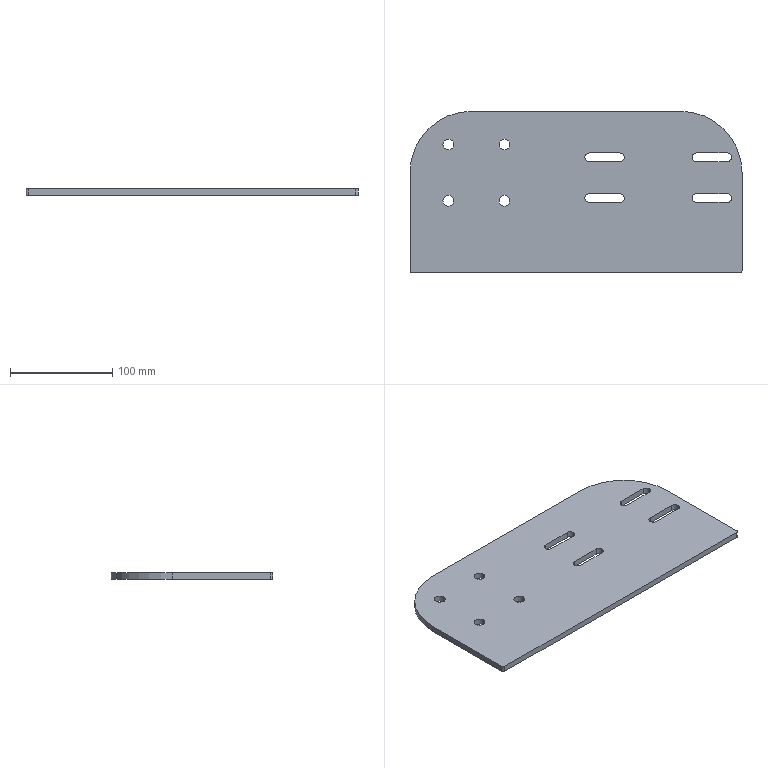Part | 1 solid | 38 faces | box 325 x 158 x 6 mm | volume 289259 mm3 | cylinder 24 | plane 14 | commonest cylinder face diameters 8.5 x12 10.5 x8 4 x2 120 x2
STEP:
#1=CARTESIAN_POINT('',(152.25,-25.,-3.));
#2=VERTEX_POINT('',#1);
#3=CARTESIAN_POINT('',(148.,-20.75,-3.));
#4=VERTEX_POINT('',#3);
#5=CARTESIAN_POINT('',(148.,-25.,-3.));
#6=DIRECTION('',(0.,0.,1.));
#7=DIRECTION('',(1.,0.,0.));
#8=AXIS2_PLACEMENT_3D('',#5,#6,#7);
#9=CIRCLE('',#8,4.25);
#10=EDGE_CURVE('',#2,#4,#9,.T.);
#11=ORIENTED_EDGE('',*,*,#10,.F.);
#12=CARTESIAN_POINT('',(152.25,-25.,3.));
#13=VERTEX_POINT('',#12);
#14=CARTESIAN_POINT('',(152.25,-25.,-3.));
#15=DIRECTION('',(0.,0.,1.));
#16=VECTOR('',#15,1000.);
#17=LINE('',#14,#16);
#18=EDGE_CURVE('',#2,#13,#17,.T.);
#19=ORIENTED_EDGE('',*,*,#18,.T.);
#20=CARTESIAN_POINT('',(148.,-20.75,3.));
#21=VERTEX_POINT('',#20);
#22=CARTESIAN_POINT('',(148.,-25.,3.));
#23=DIRECTION('',(0.,0.,1.));
#24=DIRECTION('',(1.,0.,0.));
#25=AXIS2_PLACEMENT_3D('',#22,#23,#24);
#26=CIRCLE('',#25,4.25);
#27=EDGE_CURVE('',#13,#21,#26,.T.);
#28=ORIENTED_EDGE('',*,*,#27,.T.);
#29=CARTESIAN_POINT('',(148.,-20.75,-3.));
#30=DIRECTION('',(0.,0.,1.));
#31=VECTOR('',#30,1000.);
#32=LINE('',#29,#31);
#33=EDGE_CURVE('',#4,#21,#32,.T.);
#34=ORIENTED_EDGE('',*,*,#33,.F.);
#35=EDGE_LOOP('',(#11,#19,#28,#34));
#36=FACE_OUTER_BOUND('',#35,.T.);
#37=CARTESIAN_POINT('',(148.,-25.,-3.));
#38=DIRECTION('',(0.,0.,1.));
#39=DIRECTION('',(1.,0.,0.));
#40=AXIS2_PLACEMENT_3D('',#37,#38,#39);
#41=CYLINDRICAL_SURFACE('',#40,4.25);
#42=ADVANCED_FACE('',(#36),#41,.F.);
#43=CARTESIAN_POINT('',(47.25,-25.,-3.));
#44=VERTEX_POINT('',#43);
#45=CARTESIAN_POINT('',(43.,-20.75,-3.));
#46=VERTEX_POINT('',#45);
#47=CARTESIAN_POINT('',(43.,-25.,-3.));
#48=DIRECTION('',(0.,0.,1.));
#49=DIRECTION('',(1.,0.,0.));
#50=AXIS2_PLACEMENT_3D('',#47,#48,#49);
#51=CIRCLE('',#50,4.25);
#52=EDGE_CURVE('',#44,#46,#51,.T.);
#53=ORIENTED_EDGE('',*,*,#52,.F.);
#54=CARTESIAN_POINT('',(47.25,-25.,3.));
#55=VERTEX_POINT('',#54);
#56=CARTESIAN_POINT('',(47.25,-25.,-3.));
#57=DIRECTION('',(0.,0.,1.));
#58=VECTOR('',#57,1000.);
#59=LINE('',#56,#58);
#60=EDGE_CURVE('',#44,#55,#59,.T.);
#61=ORIENTED_EDGE('',*,*,#60,.T.);
#62=CARTESIAN_POINT('',(43.,-20.75,3.));
#63=VERTEX_POINT('',#62);
#64=CARTESIAN_POINT('',(43.,-25.,3.));
#65=DIRECTION('',(0.,0.,1.));
#66=DIRECTION('',(1.,0.,0.));
#67=AXIS2_PLACEMENT_3D('',#64,#65,#66);
#68=CIRCLE('',#67,4.25);
#69=EDGE_CURVE('',#55,#63,#68,.T.);
#70=ORIENTED_EDGE('',*,*,#69,.T.);
#71=CARTESIAN_POINT('',(43.,-20.75,-3.));
#72=DIRECTION('',(0.,0.,1.));
#73=VECTOR('',#72,1000.);
#74=LINE('',#71,#73);
#75=EDGE_CURVE('',#46,#63,#74,.T.);
#76=ORIENTED_EDGE('',*,*,#75,.F.);
#77=EDGE_LOOP('',(#53,#61,#70,#76));
#78=FACE_OUTER_BOUND('',#77,.T.);
#79=CARTESIAN_POINT('',(43.,-25.,-3.));
#80=DIRECTION('',(0.,0.,1.));
#81=DIRECTION('',(1.,0.,0.));
#82=AXIS2_PLACEMENT_3D('',#79,#80,#81);
#83=CYLINDRICAL_SURFACE('',#82,4.25);
#84=ADVANCED_FACE('',(#78),#83,.F.);
#85=CARTESIAN_POINT('',(152.25,15.,-3.));
#86=VERTEX_POINT('',#85);
#87=CARTESIAN_POINT('',(148.,19.25,-3.));
#88=VERTEX_POINT('',#87);
#89=CARTESIAN_POINT('',(148.,15.,-3.));
#90=DIRECTION('',(0.,0.,1.));
#91=DIRECTION('',(1.,0.,0.));
#92=AXIS2_PLACEMENT_3D('',#89,#90,#91);
#93=CIRCLE('',#92,4.25);
#94=EDGE_CURVE('',#86,#88,#93,.T.);
#95=ORIENTED_EDGE('',*,*,#94,.F.);
#96=CARTESIAN_POINT('',(152.25,15.,3.));
#97=VERTEX_POINT('',#96);
#98=CARTESIAN_POINT('',(152.25,15.,-3.));
#99=DIRECTION('',(0.,0.,1.));
#100=VECTOR('',#99,1000.);
#101=LINE('',#98,#100);
#102=EDGE_CURVE('',#86,#97,#101,.T.);
#103=ORIENTED_EDGE('',*,*,#102,.T.);
#104=CARTESIAN_POINT('',(148.,19.25,3.));
#105=VERTEX_POINT('',#104);
#106=CARTESIAN_POINT('',(148.,15.,3.));
#107=DIRECTION('',(0.,0.,1.));
#108=DIRECTION('',(1.,0.,0.));
#109=AXIS2_PLACEMENT_3D('',#106,#107,#108);
#110=CIRCLE('',#109,4.25);
#111=EDGE_CURVE('',#97,#105,#110,.T.);
#112=ORIENTED_EDGE('',*,*,#111,.T.);
#113=CARTESIAN_POINT('',(148.,19.25,-3.));
#114=DIRECTION('',(0.,0.,1.));
#115=VECTOR('',#114,1000.);
#116=LINE('',#113,#115);
#117=EDGE_CURVE('',#88,#105,#116,.T.);
#118=ORIENTED_EDGE('',*,*,#117,.F.);
#119=EDGE_LOOP('',(#95,#103,#112,#118));
#120=FACE_OUTER_BOUND('',#119,.T.);
#121=CARTESIAN_POINT('',(148.,15.,-3.));
#122=DIRECTION('',(0.,0.,1.));
#123=DIRECTION('',(1.,0.,0.));
#124=AXIS2_PLACEMENT_3D('',#121,#122,#123);
#125=CYLINDRICAL_SURFACE('',#124,4.25);
#126=ADVANCED_FACE('',(#120),#125,.F.);
#127=CARTESIAN_POINT('',(47.25,15.,-3.));
#128=VERTEX_POINT('',#127);
#129=CARTESIAN_POINT('',(43.,19.25,-3.));
#130=VERTEX_POINT('',#129);
#131=CARTESIAN_POINT('',(43.,15.,-3.));
#132=DIRECTION('',(0.,0.,1.));
#133=DIRECTION('',(1.,0.,0.));
#134=AXIS2_PLACEMENT_3D('',#131,#132,#133);
#135=CIRCLE('',#134,4.25);
#136=EDGE_CURVE('',#128,#130,#135,.T.);
#137=ORIENTED_EDGE('',*,*,#136,.F.);
#138=CARTESIAN_POINT('',(47.25,15.,3.));
#139=VERTEX_POINT('',#138);
#140=CARTESIAN_POINT('',(47.25,15.,-3.));
#141=DIRECTION('',(0.,0.,1.));
#142=VECTOR('',#141,1000.);
#143=LINE('',#140,#142);
#144=EDGE_CURVE('',#128,#139,#143,.T.);
#145=ORIENTED_EDGE('',*,*,#144,.T.);
#146=CARTESIAN_POINT('',(43.,19.25,3.));
#147=VERTEX_POINT('',#146);
#148=CARTESIAN_POINT('',(43.,15.,3.));
#149=DIRECTION('',(0.,0.,1.));
#150=DIRECTION('',(1.,0.,0.));
#151=AXIS2_PLACEMENT_3D('',#148,#149,#150);
#152=CIRCLE('',#151,4.25);
#153=EDGE_CURVE('',#139,#147,#152,.T.);
#154=ORIENTED_EDGE('',*,*,#153,.T.);
#155=CARTESIAN_POINT('',(43.,19.25,-3.));
#156=DIRECTION('',(0.,0.,1.));
#157=VECTOR('',#156,1000.);
#158=LINE('',#155,#157);
#159=EDGE_CURVE('',#130,#147,#158,.T.);
#160=ORIENTED_EDGE('',*,*,#159,.F.);
#161=EDGE_LOOP('',(#137,#145,#154,#160));
#162=FACE_OUTER_BOUND('',#161,.T.);
#163=CARTESIAN_POINT('',(43.,15.,-3.));
#164=DIRECTION('',(0.,0.,1.));
#165=DIRECTION('',(1.,0.,0.));
#166=AXIS2_PLACEMENT_3D('',#163,#164,#165);
#167=CYLINDRICAL_SURFACE('',#166,4.25);
#168=ADVANCED_FACE('',(#162),#167,.F.);
#169=CARTESIAN_POINT('',(-75.25,-27.5,-3.));
#170=VERTEX_POINT('',#169);
#171=CARTESIAN_POINT('',(-64.75,-27.5,-3.));
#172=VERTEX_POINT('',#171);
#173=CARTESIAN_POINT('',(-70.,-27.5,-3.));
#174=DIRECTION('',(0.,0.,1.));
#175=DIRECTION('',(1.,0.,0.));
#176=AXIS2_PLACEMENT_3D('',#173,#174,#175);
#177=CIRCLE('',#176,5.25);
#178=EDGE_CURVE('',#170,#172,#177,.T.);
#179=ORIENTED_EDGE('',*,*,#178,.F.);
#180=CARTESIAN_POINT('',(-75.25,-27.5,3.));
#181=VERTEX_POINT('',#180);
#182=CARTESIAN_POINT('',(-75.25,-27.5,-3.));
#183=DIRECTION('',(0.,0.,1.));
#184=VECTOR('',#183,1000.);
#185=LINE('',#182,#184);
#186=EDGE_CURVE('',#170,#181,#185,.T.);
#187=ORIENTED_EDGE('',*,*,#186,.T.);
#188=CARTESIAN_POINT('',(-64.75,-27.5,3.));
#189=VERTEX_POINT('',#188);
#190=CARTESIAN_POINT('',(-70.,-27.5,3.));
#191=DIRECTION('',(0.,0.,1.));
#192=DIRECTION('',(1.,0.,0.));
#193=AXIS2_PLACEMENT_3D('',#190,#191,#192);
#194=CIRCLE('',#193,5.25);
#195=EDGE_CURVE('',#181,#189,#194,.T.);
#196=ORIENTED_EDGE('',*,*,#195,.T.);
#197=CARTESIAN_POINT('',(-64.75,-27.5,-3.));
#198=DIRECTION('',(0.,0.,1.));
#199=VECTOR('',#198,1000.);
#200=LINE('',#197,#199);
#201=EDGE_CURVE('',#172,#189,#200,.T.);
#202=ORIENTED_EDGE('',*,*,#201,.F.);
#203=EDGE_LOOP('',(#179,#187,#196,#202));
#204=FACE_OUTER_BOUND('',#203,.T.);
#205=CARTESIAN_POINT('',(-70.,-27.5,-3.));
#206=DIRECTION('',(0.,0.,1.));
#207=DIRECTION('',(1.,0.,0.));
#208=AXIS2_PLACEMENT_3D('',#205,#206,#207);
#209=CYLINDRICAL_SURFACE('',#208,5.25);
#210=ADVANCED_FACE('',(#204),#209,.F.);
#211=CARTESIAN_POINT('',(-130.25,-27.5,-3.));
#212=VERTEX_POINT('',#211);
#213=CARTESIAN_POINT('',(-119.75,-27.5,-3.));
#214=VERTEX_POINT('',#213);
#215=CARTESIAN_POINT('',(-125.,-27.5,-3.));
#216=DIRECTION('',(0.,0.,1.));
#217=DIRECTION('',(1.,0.,0.));
#218=AXIS2_PLACEMENT_3D('',#215,#216,#217);
#219=CIRCLE('',#218,5.25);
#220=EDGE_CURVE('',#212,#214,#219,.T.);
#221=ORIENTED_EDGE('',*,*,#220,.F.);
#222=CARTESIAN_POINT('',(-130.25,-27.5,3.));
#223=VERTEX_POINT('',#222);
#224=CARTESIAN_POINT('',(-130.25,-27.5,-3.));
#225=DIRECTION('',(0.,0.,1.));
#226=VECTOR('',#225,1000.);
#227=LINE('',#224,#226);
#228=EDGE_CURVE('',#212,#223,#227,.T.);
#229=ORIENTED_EDGE('',*,*,#228,.T.);
#230=CARTESIAN_POINT('',(-119.75,-27.5,3.));
#231=VERTEX_POINT('',#230);
#232=CARTESIAN_POINT('',(-125.,-27.5,3.));
#233=DIRECTION('',(0.,0.,1.));
#234=DIRECTION('',(1.,0.,0.));
#235=AXIS2_PLACEMENT_3D('',#232,#233,#234);
#236=CIRCLE('',#235,5.25);
#237=EDGE_CURVE('',#223,#231,#236,.T.);
#238=ORIENTED_EDGE('',*,*,#237,.T.);
#239=CARTESIAN_POINT('',(-119.75,-27.5,-3.));
#240=DIRECTION('',(0.,0.,1.));
#241=VECTOR('',#240,1000.);
#242=LINE('',#239,#241);
#243=EDGE_CURVE('',#214,#231,#242,.T.);
#244=ORIENTED_EDGE('',*,*,#243,.F.);
#245=EDGE_LOOP('',(#221,#229,#238,#244));
#246=FACE_OUTER_BOUND('',#245,.T.);
#247=CARTESIAN_POINT('',(-125.,-27.5,-3.));
#248=DIRECTION('',(0.,0.,1.));
#249=DIRECTION('',(1.,0.,0.));
#250=AXIS2_PLACEMENT_3D('',#247,#248,#249);
#251=CYLINDRICAL_SURFACE('',#250,5.25);
#252=ADVANCED_FACE('',(#246),#251,.F.);
#253=CARTESIAN_POINT('',(-75.25,27.5,-3.));
#254=VERTEX_POINT('',#253);
#255=CARTESIAN_POINT('',(-64.75,27.5,-3.));
#256=VERTEX_POINT('',#255);
#257=CARTESIAN_POINT('',(-70.,27.5,-3.));
#258=DIRECTION('',(0.,0.,1.));
#259=DIRECTION('',(1.,0.,0.));
#260=AXIS2_PLACEMENT_3D('',#257,#258,#259);
#261=CIRCLE('',#260,5.25);
#262=EDGE_CURVE('',#254,#256,#261,.T.);
#263=ORIENTED_EDGE('',*,*,#262,.F.);
#264=CARTESIAN_POINT('',(-75.25,27.5,3.));
#265=VERTEX_POINT('',#264);
#266=CARTESIAN_POINT('',(-75.25,27.5,-3.));
#267=DIRECTION('',(0.,0.,1.));
#268=VECTOR('',#267,1000.);
#269=LINE('',#266,#268);
#270=EDGE_CURVE('',#254,#265,#269,.T.);
#271=ORIENTED_EDGE('',*,*,#270,.T.);
#272=CARTESIAN_POINT('',(-64.75,27.5,3.));
#273=VERTEX_POINT('',#272);
#274=CARTESIAN_POINT('',(-70.,27.5,3.));
#275=DIRECTION('',(0.,0.,1.));
#276=DIRECTION('',(1.,0.,0.));
#277=AXIS2_PLACEMENT_3D('',#274,#275,#276);
#278=CIRCLE('',#277,5.25);
#279=EDGE_CURVE('',#265,#273,#278,.T.);
#280=ORIENTED_EDGE('',*,*,#279,.T.);
#281=CARTESIAN_POINT('',(-64.75,27.5,-3.));
#282=DIRECTION('',(0.,0.,1.));
#283=VECTOR('',#282,1000.);
#284=LINE('',#281,#283);
#285=EDGE_CURVE('',#256,#273,#284,.T.);
#286=ORIENTED_EDGE('',*,*,#285,.F.);
#287=EDGE_LOOP('',(#263,#271,#280,#286));
#288=FACE_OUTER_BOUND('',#287,.T.);
#289=CARTESIAN_POINT('',(-70.,27.5,-3.));
#290=DIRECTION('',(0.,0.,1.));
#291=DIRECTION('',(1.,0.,0.));
#292=AXIS2_PLACEMENT_3D('',#289,#290,#291);
#293=CYLINDRICAL_SURFACE('',#292,5.25);
#294=ADVANCED_FACE('',(#288),#293,.F.);
#295=CARTESIAN_POINT('',(-130.25,27.5,-3.));
#296=VERTEX_POINT('',#295);
#297=CARTESIAN_POINT('',(-119.75,27.5,-3.));
#298=VERTEX_POINT('',#297);
#299=CARTESIAN_POINT('',(-125.,27.5,-3.));
#300=DIRECTION('',(0.,0.,1.));
#301=DIRECTION('',(1.,0.,0.));
#302=AXIS2_PLACEMENT_3D('',#299,#300,#301);
#303=CIRCLE('',#302,5.25);
#304=EDGE_CURVE('',#296,#298,#303,.T.);
#305=ORIENTED_EDGE('',*,*,#304,.F.);
#306=CARTESIAN_POINT('',(-130.25,27.5,3.));
#307=VERTEX_POINT('',#306);
#308=CARTESIAN_POINT('',(-130.25,27.5,-3.));
#309=DIRECTION('',(0.,0.,1.));
#310=VECTOR('',#309,1000.);
#311=LINE('',#308,#310);
#312=EDGE_CURVE('',#296,#307,#311,.T.);
#313=ORIENTED_EDGE('',*,*,#312,.T.);
#314=CARTESIAN_POINT('',(-119.75,27.5,3.));
#315=VERTEX_POINT('',#314);
#316=CARTESIAN_POINT('',(-125.,27.5,3.));
#317=DIRECTION('',(0.,0.,1.));
#318=DIRECTION('',(1.,0.,0.));
#319=AXIS2_PLACEMENT_3D('',#316,#317,#318);
#320=CIRCLE('',#319,5.25);
#321=EDGE_CURVE('',#307,#315,#320,.T.);
#322=ORIENTED_EDGE('',*,*,#321,.T.);
#323=CARTESIAN_POINT('',(-119.75,27.5,-3.));
#324=DIRECTION('',(0.,0.,1.));
#325=VECTOR('',#324,1000.);
#326=LINE('',#323,#325);
#327=EDGE_CURVE('',#298,#315,#326,.T.);
#328=ORIENTED_EDGE('',*,*,#327,.F.);
#329=EDGE_LOOP('',(#305,#313,#322,#328));
#330=FACE_OUTER_BOUND('',#329,.T.);
#331=CARTESIAN_POINT('',(-125.,27.5,-3.));
#332=DIRECTION('',(0.,0.,1.));
#333=DIRECTION('',(1.,0.,0.));
#334=AXIS2_PLACEMENT_3D('',#331,#332,#333);
#335=CYLINDRICAL_SURFACE('',#334,5.25);
#336=ADVANCED_FACE('',(#330),#335,.F.);
#337=CARTESIAN_POINT('',(-162.5,0.,-3.));
#338=VERTEX_POINT('',#337);
#339=CARTESIAN_POINT('',(-162.5,0.,3.));
#340=VERTEX_POINT('',#339);
#341=CARTESIAN_POINT('',(-162.5,0.,-3.));
#342=DIRECTION('',(0.,0.,1.));
#343=VECTOR('',#342,1000.);
#344=LINE('',#341,#343);
#345=EDGE_CURVE('',#338,#340,#344,.T.);
#346=ORIENTED_EDGE('',*,*,#345,.T.);
#347=CARTESIAN_POINT('',(-102.5,60.,3.));
#348=VERTEX_POINT('',#347);
#349=CARTESIAN_POINT('',(-102.5,0.,3.));
#350=DIRECTION('',(0.,0.,1.));
#351=DIRECTION('',(1.,0.,0.));
#352=AXIS2_PLACEMENT_3D('',#349,#350,#351);
#353=CIRCLE('',#352,60.);
#354=EDGE_CURVE('',#348,#340,#353,.T.);
#355=ORIENTED_EDGE('',*,*,#354,.F.);
#356=CARTESIAN_POINT('',(-102.5,60.,-3.));
#357=VERTEX_POINT('',#356);
#358=CARTESIAN_POINT('',(-102.5,60.,3.));
#359=DIRECTION('',(0.,0.,-1.));
#360=VECTOR('',#359,1000.);
#361=LINE('',#358,#360);
#362=EDGE_CURVE('',#348,#357,#361,.T.);
#363=ORIENTED_EDGE('',*,*,#362,.T.);
#364=CARTESIAN_POINT('',(-102.5,0.,-3.));
#365=DIRECTION('',(0.,0.,1.));
#366=DIRECTION('',(1.,0.,0.));
#367=AXIS2_PLACEMENT_3D('',#364,#365,#366);
#368=CIRCLE('',#367,60.);
#369=EDGE_CURVE('',#357,#338,#368,.T.);
#370=ORIENTED_EDGE('',*,*,#369,.T.);
#371=EDGE_LOOP('',(#346,#355,#363,#370));
#372=FACE_OUTER_BOUND('',#371,.T.);
#373=CARTESIAN_POINT('',(-102.5,0.,3.));
#374=DIRECTION('',(0.,0.,-1.));
#375=DIRECTION('',(-1.,0.,0.));
#376=AXIS2_PLACEMENT_3D('',#373,#374,#375);
#377=CYLINDRICAL_SURFACE('',#376,60.);
#378=ADVANCED_FACE('',(#372),#377,.T.);
#379=CARTESIAN_POINT('',(162.5,0.,3.));
#380=VERTEX_POINT('',#379);
#381=CARTESIAN_POINT('',(102.5,60.,3.));
#382=VERTEX_POINT('',#381);
#383=CARTESIAN_POINT('',(102.5,0.,3.));
#384=DIRECTION('',(0.,0.,1.));
#385=DIRECTION('',(1.,0.,0.));
#386=AXIS2_PLACEMENT_3D('',#383,#384,#385);
#387=CIRCLE('',#386,60.);
#388=EDGE_CURVE('',#380,#382,#387,.T.);
#389=ORIENTED_EDGE('',*,*,#388,.F.);
#390=CARTESIAN_POINT('',(162.5,0.,-3.));
#391=VERTEX_POINT('',#390);
#392=CARTESIAN_POINT('',(162.5,0.,-3.));
#393=DIRECTION('',(0.,0.,1.));
#394=VECTOR('',#393,1000.);
#395=LINE('',#392,#394);
#396=EDGE_CURVE('',#391,#380,#395,.T.);
#397=ORIENTED_EDGE('',*,*,#396,.F.);
#398=CARTESIAN_POINT('',(102.5,60.,-3.));
#399=VERTEX_POINT('',#398);
#400=CARTESIAN_POINT('',(102.5,0.,-3.));
#401=DIRECTION('',(0.,0.,1.));
#402=DIRECTION('',(1.,0.,0.));
#403=AXIS2_PLACEMENT_3D('',#400,#401,#402);
#404=CIRCLE('',#403,60.);
#405=EDGE_CURVE('',#391,#399,#404,.T.);
#406=ORIENTED_EDGE('',*,*,#405,.T.);
#407=CARTESIAN_POINT('',(102.5,60.,3.));
#408=DIRECTION('',(0.,0.,-1.));
#409=VECTOR('',#408,1000.);
#410=LINE('',#407,#409);
#411=EDGE_CURVE('',#382,#399,#410,.T.);
#412=ORIENTED_EDGE('',*,*,#411,.F.);
#413=EDGE_LOOP('',(#389,#397,#406,#412));
#414=FACE_OUTER_BOUND('',#413,.T.);
#415=CARTESIAN_POINT('',(102.5,0.,3.));
#416=DIRECTION('',(0.,0.,-1.));
#417=DIRECTION('',(-1.,0.,0.));
#418=AXIS2_PLACEMENT_3D('',#415,#416,#417);
#419=CYLINDRICAL_SURFACE('',#418,60.);
#420=ADVANCED_FACE('',(#414),#419,.T.);
#421=CARTESIAN_POINT('',(-102.5,60.,-3.));
#422=DIRECTION('',(-1.,0.,0.));
#423=VECTOR('',#422,1000.);
#424=LINE('',#421,#423);
#425=EDGE_CURVE('',#399,#357,#424,.T.);
#426=ORIENTED_EDGE('',*,*,#425,.T.);
#427=ORIENTED_EDGE('',*,*,#362,.F.);
#428=CARTESIAN_POINT('',(-102.5,60.,3.));
#429=DIRECTION('',(-1.,0.,0.));
#430=VECTOR('',#429,1000.);
#431=LINE('',#428,#430);
#432=EDGE_CURVE('',#382,#348,#431,.T.);
#433=ORIENTED_EDGE('',*,*,#432,.F.);
#434=ORIENTED_EDGE('',*,*,#411,.T.);
#435=EDGE_LOOP('',(#426,#427,#433,#434));
#436=FACE_OUTER_BOUND('',#435,.T.);
#437=CARTESIAN_POINT('',(-102.5,60.,3.));
#438=DIRECTION('',(0.,-1.,0.));
#439=DIRECTION('',(1.,0.,0.));
#440=AXIS2_PLACEMENT_3D('',#437,#438,#439);
#441=PLANE('',#440);
#442=ADVANCED_FACE('',(#436),#441,.F.);
#443=CARTESIAN_POINT('',(118.,-20.75,3.));
#444=VERTEX_POINT('',#443);
#445=CARTESIAN_POINT('',(118.,-29.25,3.));
#446=VERTEX_POINT('',#445);
#447=CARTESIAN_POINT('',(118.,-25.,3.));
#448=DIRECTION('',(0.,0.,1.));
#449=DIRECTION('',(1.,0.,0.));
#450=AXIS2_PLACEMENT_3D('',#447,#448,#449);
#451=CIRCLE('',#450,4.25);
#452=EDGE_CURVE('',#444,#446,#451,.T.);
#453=ORIENTED_EDGE('',*,*,#452,.F.);
#454=CARTESIAN_POINT('',(118.,-20.75,3.));
#455=DIRECTION('',(-1.,0.,0.));
#456=VECTOR('',#455,1000.);
#457=LINE('',#454,#456);
#458=EDGE_CURVE('',#21,#444,#457,.T.);
#459=ORIENTED_EDGE('',*,*,#458,.F.);
#460=ORIENTED_EDGE('',*,*,#27,.F.);
#461=CARTESIAN_POINT('',(148.,-29.25,3.));
#462=VERTEX_POINT('',#461);
#463=CARTESIAN_POINT('',(148.,-25.,3.));
#464=DIRECTION('',(0.,0.,1.));
#465=DIRECTION('',(1.,0.,0.));
#466=AXIS2_PLACEMENT_3D('',#463,#464,#465);
#467=CIRCLE('',#466,4.25);
#468=EDGE_CURVE('',#462,#13,#467,.T.);
#469=ORIENTED_EDGE('',*,*,#468,.F.);
#470=CARTESIAN_POINT('',(118.,-29.25,3.));
#471=DIRECTION('',(1.,0.,0.));
#472=VECTOR('',#471,1000.);
#473=LINE('',#470,#472);
#474=EDGE_CURVE('',#446,#462,#473,.T.);
#475=ORIENTED_EDGE('',*,*,#474,.F.);
#476=EDGE_LOOP('',(#453,#459,#460,#469,#475));
#477=FACE_BOUND('',#476,.T.);
#478=CARTESIAN_POINT('',(13.,-20.75,3.));
#479=VERTEX_POINT('',#478);
#480=CARTESIAN_POINT('',(13.,-29.25,3.));
#481=VERTEX_POINT('',#480);
#482=CARTESIAN_POINT('',(13.,-25.,3.));
#483=DIRECTION('',(0.,0.,1.));
#484=DIRECTION('',(1.,0.,0.));
#485=AXIS2_PLACEMENT_3D('',#482,#483,#484);
#486=CIRCLE('',#485,4.25);
#487=EDGE_CURVE('',#479,#481,#486,.T.);
#488=ORIENTED_EDGE('',*,*,#487,.F.);
#489=CARTESIAN_POINT('',(13.,-20.75,3.));
#490=DIRECTION('',(-1.,0.,0.));
#491=VECTOR('',#490,1000.);
#492=LINE('',#489,#491);
#493=EDGE_CURVE('',#63,#479,#492,.T.);
#494=ORIENTED_EDGE('',*,*,#493,.F.);
#495=ORIENTED_EDGE('',*,*,#69,.F.);
#496=CARTESIAN_POINT('',(43.,-29.25,3.));
#497=VERTEX_POINT('',#496);
#498=CARTESIAN_POINT('',(43.,-25.,3.));
#499=DIRECTION('',(0.,0.,1.));
#500=DIRECTION('',(1.,0.,0.));
#501=AXIS2_PLACEMENT_3D('',#498,#499,#500);
#502=CIRCLE('',#501,4.25);
#503=EDGE_CURVE('',#497,#55,#502,.T.);
#504=ORIENTED_EDGE('',*,*,#503,.F.);
#505=CARTESIAN_POINT('',(13.,-29.25,3.));
#506=DIRECTION('',(1.,0.,0.));
#507=VECTOR('',#506,1000.);
#508=LINE('',#505,#507);
#509=EDGE_CURVE('',#481,#497,#508,.T.);
#510=ORIENTED_EDGE('',*,*,#509,.F.);
#511=EDGE_LOOP('',(#488,#494,#495,#504,#510));
#512=FACE_BOUND('',#511,.T.);
#513=CARTESIAN_POINT('',(118.,19.25,3.));
#514=VERTEX_POINT('',#513);
#515=CARTESIAN_POINT('',(118.,10.75,3.));
#516=VERTEX_POINT('',#515);
#517=CARTESIAN_POINT('',(118.,15.,3.));
#518=DIRECTION('',(0.,0.,1.));
#519=DIRECTION('',(1.,0.,0.));
#520=AXIS2_PLACEMENT_3D('',#517,#518,#519);
#521=CIRCLE('',#520,4.25);
#522=EDGE_CURVE('',#514,#516,#521,.T.);
#523=ORIENTED_EDGE('',*,*,#522,.F.);
#524=CARTESIAN_POINT('',(118.,19.25,3.));
#525=DIRECTION('',(-1.,0.,0.));
#526=VECTOR('',#525,1000.);
#527=LINE('',#524,#526);
#528=EDGE_CURVE('',#105,#514,#527,.T.);
#529=ORIENTED_EDGE('',*,*,#528,.F.);
#530=ORIENTED_EDGE('',*,*,#111,.F.);
#531=CARTESIAN_POINT('',(148.,10.75,3.));
#532=VERTEX_POINT('',#531);
#533=CARTESIAN_POINT('',(148.,15.,3.));
#534=DIRECTION('',(0.,0.,1.));
#535=DIRECTION('',(1.,0.,0.));
#536=AXIS2_PLACEMENT_3D('',#533,#534,#535);
#537=CIRCLE('',#536,4.25);
#538=EDGE_CURVE('',#532,#97,#537,.T.);
#539=ORIENTED_EDGE('',*,*,#538,.F.);
#540=CARTESIAN_POINT('',(118.,10.75,3.));
#541=DIRECTION('',(1.,0.,0.));
#542=VECTOR('',#541,1000.);
#543=LINE('',#540,#542);
#544=EDGE_CURVE('',#516,#532,#543,.T.);
#545=ORIENTED_EDGE('',*,*,#544,.F.);
#546=EDGE_LOOP('',(#523,#529,#530,#539,#545));
#547=FACE_BOUND('',#546,.T.);
#548=CARTESIAN_POINT('',(13.,19.25,3.));
#549=VERTEX_POINT('',#548);
#550=CARTESIAN_POINT('',(13.,10.75,3.));
#551=VERTEX_POINT('',#550);
#552=CARTESIAN_POINT('',(13.,15.,3.));
#553=DIRECTION('',(0.,0.,1.));
#554=DIRECTION('',(1.,0.,0.));
#555=AXIS2_PLACEMENT_3D('',#552,#553,#554);
#556=CIRCLE('',#555,4.25);
#557=EDGE_CURVE('',#549,#551,#556,.T.);
#558=ORIENTED_EDGE('',*,*,#557,.F.);
#559=CARTESIAN_POINT('',(13.,19.25,3.));
#560=DIRECTION('',(-1.,0.,0.));
#561=VECTOR('',#560,1000.);
#562=LINE('',#559,#561);
#563=EDGE_CURVE('',#147,#549,#562,.T.);
#564=ORIENTED_EDGE('',*,*,#563,.F.);
#565=ORIENTED_EDGE('',*,*,#153,.F.);
#566=CARTESIAN_POINT('',(43.,10.75,3.));
#567=VERTEX_POINT('',#566);
#568=CARTESIAN_POINT('',(43.,15.,3.));
#569=DIRECTION('',(0.,0.,1.));
#570=DIRECTION('',(1.,0.,0.));
#571=AXIS2_PLACEMENT_3D('',#568,#569,#570);
#572=CIRCLE('',#571,4.25);
#573=EDGE_CURVE('',#567,#139,#572,.T.);
#574=ORIENTED_EDGE('',*,*,#573,.F.);
#575=CARTESIAN_POINT('',(13.,10.75,3.));
#576=DIRECTION('',(1.,0.,0.));
#577=VECTOR('',#576,1000.);
#578=LINE('',#575,#577);
#579=EDGE_CURVE('',#551,#567,#578,.T.);
#580=ORIENTED_EDGE('',*,*,#579,.F.);
#581=EDGE_LOOP('',(#558,#564,#565,#574,#580));
#582=FACE_BOUND('',#581,.T.);
#583=CARTESIAN_POINT('',(-70.,-27.5,3.));
#584=DIRECTION('',(0.,0.,1.));
#585=DIRECTION('',(1.,0.,0.));
#586=AXIS2_PLACEMENT_3D('',#583,#584,#585);
#587=CIRCLE('',#586,5.25);
#588=EDGE_CURVE('',#189,#181,#587,.T.);
#589=ORIENTED_EDGE('',*,*,#588,.F.);
#590=ORIENTED_EDGE('',*,*,#195,.F.);
#591=EDGE_LOOP('',(#589,#590));
#592=FACE_BOUND('',#591,.T.);
#593=CARTESIAN_POINT('',(-125.,-27.5,3.));
#594=DIRECTION('',(0.,0.,1.));
#595=DIRECTION('',(1.,0.,0.));
#596=AXIS2_PLACEMENT_3D('',#593,#594,#595);
#597=CIRCLE('',#596,5.25);
#598=EDGE_CURVE('',#231,#223,#597,.T.);
#599=ORIENTED_EDGE('',*,*,#598,.F.);
#600=ORIENTED_EDGE('',*,*,#237,.F.);
#601=EDGE_LOOP('',(#599,#600));
#602=FACE_BOUND('',#601,.T.);
#603=CARTESIAN_POINT('',(-70.,27.5,3.));
#604=DIRECTION('',(0.,0.,1.));
#605=DIRECTION('',(1.,0.,0.));
#606=AXIS2_PLACEMENT_3D('',#603,#604,#605);
#607=CIRCLE('',#606,5.25);
#608=EDGE_CURVE('',#273,#265,#607,.T.);
#609=ORIENTED_EDGE('',*,*,#608,.F.);
#610=ORIENTED_EDGE('',*,*,#279,.F.);
#611=EDGE_LOOP('',(#609,#610));
#612=FACE_BOUND('',#611,.T.);
#613=CARTESIAN_POINT('',(-125.,27.5,3.));
#614=DIRECTION('',(0.,0.,1.));
#615=DIRECTION('',(1.,0.,0.));
#616=AXIS2_PLACEMENT_3D('',#613,#614,#615);
#617=CIRCLE('',#616,5.25);
#618=EDGE_CURVE('',#315,#307,#617,.T.);
#619=ORIENTED_EDGE('',*,*,#618,.F.);
#620=ORIENTED_EDGE('',*,*,#321,.F.);
#621=EDGE_LOOP('',(#619,#620));
#622=FACE_BOUND('',#621,.T.);
#623=CARTESIAN_POINT('',(160.5,-98.,3.));
#624=VERTEX_POINT('',#623);
#625=CARTESIAN_POINT('',(-160.5,-98.,3.));
#626=VERTEX_POINT('',#625);
#627=CARTESIAN_POINT('',(0.,-98.,3.));
#628=DIRECTION('',(-1.,0.,0.));
#629=VECTOR('',#628,1000.);
#630=LINE('',#627,#629);
#631=EDGE_CURVE('',#624,#626,#630,.T.);
#632=ORIENTED_EDGE('',*,*,#631,.F.);
#633=CARTESIAN_POINT('',(162.5,-96.,3.));
#634=VERTEX_POINT('',#633);
#635=CARTESIAN_POINT('',(160.5,-96.,3.));
#636=DIRECTION('',(0.,0.,1.));
#637=DIRECTION('',(1.,0.,0.));
#638=AXIS2_PLACEMENT_3D('',#635,#636,#637);
#639=CIRCLE('',#638,2.);
#640=EDGE_CURVE('',#624,#634,#639,.T.);
#641=ORIENTED_EDGE('',*,*,#640,.T.);
#642=CARTESIAN_POINT('',(162.5,0.,3.));
#643=DIRECTION('',(0.,-1.,0.));
#644=VECTOR('',#643,1000.);
#645=LINE('',#642,#644);
#646=EDGE_CURVE('',#380,#634,#645,.T.);
#647=ORIENTED_EDGE('',*,*,#646,.F.);
#648=ORIENTED_EDGE('',*,*,#388,.T.);
#649=ORIENTED_EDGE('',*,*,#432,.T.);
#650=ORIENTED_EDGE('',*,*,#354,.T.);
#651=CARTESIAN_POINT('',(-162.5,-96.,3.));
#652=VERTEX_POINT('',#651);
#653=CARTESIAN_POINT('',(-162.5,0.,3.));
#654=DIRECTION('',(0.,1.,0.));
#655=VECTOR('',#654,1000.);
#656=LINE('',#653,#655);
#657=EDGE_CURVE('',#652,#340,#656,.T.);
#658=ORIENTED_EDGE('',*,*,#657,.F.);
#659=CARTESIAN_POINT('',(-160.5,-96.,3.));
#660=DIRECTION('',(0.,0.,1.));
#661=DIRECTION('',(1.,0.,0.));
#662=AXIS2_PLACEMENT_3D('',#659,#660,#661);
#663=CIRCLE('',#662,2.);
#664=EDGE_CURVE('',#652,#626,#663,.T.);
#665=ORIENTED_EDGE('',*,*,#664,.T.);
#666=EDGE_LOOP('',(#632,#641,#647,#648,#649,#650,#658,#665));
#667=FACE_OUTER_BOUND('',#666,.T.);
#668=CARTESIAN_POINT('',(-102.5,0.,3.));
#669=DIRECTION('',(0.,0.,1.));
#670=DIRECTION('',(1.,0.,0.));
#671=AXIS2_PLACEMENT_3D('',#668,#669,#670);
#672=PLANE('',#671);
#673=ADVANCED_FACE('',(#477,#512,#547,#582,#592,#602,#612,#622,#667),#672,.T.);
#674=CARTESIAN_POINT('',(118.,-20.75,-3.));
#675=VERTEX_POINT('',#674);
#676=CARTESIAN_POINT('',(118.,-20.75,-3.));
#677=DIRECTION('',(-1.,0.,0.));
#678=VECTOR('',#677,1000.);
#679=LINE('',#676,#678);
#680=EDGE_CURVE('',#4,#675,#679,.T.);
#681=ORIENTED_EDGE('',*,*,#680,.T.);
#682=CARTESIAN_POINT('',(118.,-29.25,-3.));
#683=VERTEX_POINT('',#682);
#684=CARTESIAN_POINT('',(118.,-25.,-3.));
#685=DIRECTION('',(0.,0.,1.));
#686=DIRECTION('',(1.,0.,0.));
#687=AXIS2_PLACEMENT_3D('',#684,#685,#686);
#688=CIRCLE('',#687,4.25);
#689=EDGE_CURVE('',#675,#683,#688,.T.);
#690=ORIENTED_EDGE('',*,*,#689,.T.);
#691=CARTESIAN_POINT('',(148.,-29.25,-3.));
#692=VERTEX_POINT('',#691);
#693=CARTESIAN_POINT('',(118.,-29.25,-3.));
#694=DIRECTION('',(1.,0.,0.));
#695=VECTOR('',#694,1000.);
#696=LINE('',#693,#695);
#697=EDGE_CURVE('',#683,#692,#696,.T.);
#698=ORIENTED_EDGE('',*,*,#697,.T.);
#699=CARTESIAN_POINT('',(148.,-25.,-3.));
#700=DIRECTION('',(0.,0.,1.));
#701=DIRECTION('',(1.,0.,0.));
#702=AXIS2_PLACEMENT_3D('',#699,#700,#701);
#703=CIRCLE('',#702,4.25);
#704=EDGE_CURVE('',#692,#2,#703,.T.);
#705=ORIENTED_EDGE('',*,*,#704,.T.);
#706=ORIENTED_EDGE('',*,*,#10,.T.);
#707=EDGE_LOOP('',(#681,#690,#698,#705,#706));
#708=FACE_BOUND('',#707,.T.);
#709=CARTESIAN_POINT('',(13.,-20.75,-3.));
#710=VERTEX_POINT('',#709);
#711=CARTESIAN_POINT('',(13.,-20.75,-3.));
#712=DIRECTION('',(-1.,0.,0.));
#713=VECTOR('',#712,1000.);
#714=LINE('',#711,#713);
#715=EDGE_CURVE('',#46,#710,#714,.T.);
#716=ORIENTED_EDGE('',*,*,#715,.T.);
#717=CARTESIAN_POINT('',(13.,-29.25,-3.));
#718=VERTEX_POINT('',#717);
#719=CARTESIAN_POINT('',(13.,-25.,-3.));
#720=DIRECTION('',(0.,0.,1.));
#721=DIRECTION('',(1.,0.,0.));
#722=AXIS2_PLACEMENT_3D('',#719,#720,#721);
#723=CIRCLE('',#722,4.25);
#724=EDGE_CURVE('',#710,#718,#723,.T.);
#725=ORIENTED_EDGE('',*,*,#724,.T.);
#726=CARTESIAN_POINT('',(43.,-29.25,-3.));
#727=VERTEX_POINT('',#726);
#728=CARTESIAN_POINT('',(13.,-29.25,-3.));
#729=DIRECTION('',(1.,0.,0.));
#730=VECTOR('',#729,1000.);
#731=LINE('',#728,#730);
#732=EDGE_CURVE('',#718,#727,#731,.T.);
#733=ORIENTED_EDGE('',*,*,#732,.T.);
#734=CARTESIAN_POINT('',(43.,-25.,-3.));
#735=DIRECTION('',(0.,0.,1.));
#736=DIRECTION('',(1.,0.,0.));
#737=AXIS2_PLACEMENT_3D('',#734,#735,#736);
#738=CIRCLE('',#737,4.25);
#739=EDGE_CURVE('',#727,#44,#738,.T.);
#740=ORIENTED_EDGE('',*,*,#739,.T.);
#741=ORIENTED_EDGE('',*,*,#52,.T.);
#742=EDGE_LOOP('',(#716,#725,#733,#740,#741));
#743=FACE_BOUND('',#742,.T.);
#744=CARTESIAN_POINT('',(118.,19.25,-3.));
#745=VERTEX_POINT('',#744);
#746=CARTESIAN_POINT('',(118.,19.25,-3.));
#747=DIRECTION('',(-1.,0.,0.));
#748=VECTOR('',#747,1000.);
#749=LINE('',#746,#748);
#750=EDGE_CURVE('',#88,#745,#749,.T.);
#751=ORIENTED_EDGE('',*,*,#750,.T.);
#752=CARTESIAN_POINT('',(118.,10.75,-3.));
#753=VERTEX_POINT('',#752);
#754=CARTESIAN_POINT('',(118.,15.,-3.));
#755=DIRECTION('',(0.,0.,1.));
#756=DIRECTION('',(1.,0.,0.));
#757=AXIS2_PLACEMENT_3D('',#754,#755,#756);
#758=CIRCLE('',#757,4.25);
#759=EDGE_CURVE('',#745,#753,#758,.T.);
#760=ORIENTED_EDGE('',*,*,#759,.T.);
#761=CARTESIAN_POINT('',(148.,10.75,-3.));
#762=VERTEX_POINT('',#761);
#763=CARTESIAN_POINT('',(118.,10.75,-3.));
#764=DIRECTION('',(1.,0.,0.));
#765=VECTOR('',#764,1000.);
#766=LINE('',#763,#765);
#767=EDGE_CURVE('',#753,#762,#766,.T.);
#768=ORIENTED_EDGE('',*,*,#767,.T.);
#769=CARTESIAN_POINT('',(148.,15.,-3.));
#770=DIRECTION('',(0.,0.,1.));
#771=DIRECTION('',(1.,0.,0.));
#772=AXIS2_PLACEMENT_3D('',#769,#770,#771);
#773=CIRCLE('',#772,4.25);
#774=EDGE_CURVE('',#762,#86,#773,.T.);
#775=ORIENTED_EDGE('',*,*,#774,.T.);
#776=ORIENTED_EDGE('',*,*,#94,.T.);
#777=EDGE_LOOP('',(#751,#760,#768,#775,#776));
#778=FACE_BOUND('',#777,.T.);
#779=CARTESIAN_POINT('',(13.,19.25,-3.));
#780=VERTEX_POINT('',#779);
#781=CARTESIAN_POINT('',(13.,19.25,-3.));
#782=DIRECTION('',(-1.,0.,0.));
#783=VECTOR('',#782,1000.);
#784=LINE('',#781,#783);
#785=EDGE_CURVE('',#130,#780,#784,.T.);
#786=ORIENTED_EDGE('',*,*,#785,.T.);
#787=CARTESIAN_POINT('',(13.,10.75,-3.));
#788=VERTEX_POINT('',#787);
#789=CARTESIAN_POINT('',(13.,15.,-3.));
#790=DIRECTION('',(0.,0.,1.));
#791=DIRECTION('',(1.,0.,0.));
#792=AXIS2_PLACEMENT_3D('',#789,#790,#791);
#793=CIRCLE('',#792,4.25);
#794=EDGE_CURVE('',#780,#788,#793,.T.);
#795=ORIENTED_EDGE('',*,*,#794,.T.);
#796=CARTESIAN_POINT('',(43.,10.75,-3.));
#797=VERTEX_POINT('',#796);
#798=CARTESIAN_POINT('',(13.,10.75,-3.));
#799=DIRECTION('',(1.,0.,0.));
#800=VECTOR('',#799,1000.);
#801=LINE('',#798,#800);
#802=EDGE_CURVE('',#788,#797,#801,.T.);
#803=ORIENTED_EDGE('',*,*,#802,.T.);
#804=CARTESIAN_POINT('',(43.,15.,-3.));
#805=DIRECTION('',(0.,0.,1.));
#806=DIRECTION('',(1.,0.,0.));
#807=AXIS2_PLACEMENT_3D('',#804,#805,#806);
#808=CIRCLE('',#807,4.25);
#809=EDGE_CURVE('',#797,#128,#808,.T.);
#810=ORIENTED_EDGE('',*,*,#809,.T.);
#811=ORIENTED_EDGE('',*,*,#136,.T.);
#812=EDGE_LOOP('',(#786,#795,#803,#810,#811));
#813=FACE_BOUND('',#812,.T.);
#814=CARTESIAN_POINT('',(-70.,-27.5,-3.));
#815=DIRECTION('',(0.,0.,1.));
#816=DIRECTION('',(1.,0.,0.));
#817=AXIS2_PLACEMENT_3D('',#814,#815,#816);
#818=CIRCLE('',#817,5.25);
#819=EDGE_CURVE('',#172,#170,#818,.T.);
#820=ORIENTED_EDGE('',*,*,#819,.T.);
#821=ORIENTED_EDGE('',*,*,#178,.T.);
#822=EDGE_LOOP('',(#820,#821));
#823=FACE_BOUND('',#822,.T.);
#824=CARTESIAN_POINT('',(-125.,-27.5,-3.));
#825=DIRECTION('',(0.,0.,1.));
#826=DIRECTION('',(1.,0.,0.));
#827=AXIS2_PLACEMENT_3D('',#824,#825,#826);
#828=CIRCLE('',#827,5.25);
#829=EDGE_CURVE('',#214,#212,#828,.T.);
#830=ORIENTED_EDGE('',*,*,#829,.T.);
#831=ORIENTED_EDGE('',*,*,#220,.T.);
#832=EDGE_LOOP('',(#830,#831));
#833=FACE_BOUND('',#832,.T.);
#834=CARTESIAN_POINT('',(-70.,27.5,-3.));
#835=DIRECTION('',(0.,0.,1.));
#836=DIRECTION('',(1.,0.,0.));
#837=AXIS2_PLACEMENT_3D('',#834,#835,#836);
#838=CIRCLE('',#837,5.25);
#839=EDGE_CURVE('',#256,#254,#838,.T.);
#840=ORIENTED_EDGE('',*,*,#839,.T.);
#841=ORIENTED_EDGE('',*,*,#262,.T.);
#842=EDGE_LOOP('',(#840,#841));
#843=FACE_BOUND('',#842,.T.);
#844=CARTESIAN_POINT('',(-125.,27.5,-3.));
#845=DIRECTION('',(0.,0.,1.));
#846=DIRECTION('',(1.,0.,0.));
#847=AXIS2_PLACEMENT_3D('',#844,#845,#846);
#848=CIRCLE('',#847,5.25);
#849=EDGE_CURVE('',#298,#296,#848,.T.);
#850=ORIENTED_EDGE('',*,*,#849,.T.);
#851=ORIENTED_EDGE('',*,*,#304,.T.);
#852=EDGE_LOOP('',(#850,#851));
#853=FACE_BOUND('',#852,.T.);
#854=CARTESIAN_POINT('',(162.5,-96.,-3.));
#855=VERTEX_POINT('',#854);
#856=CARTESIAN_POINT('',(162.5,0.,-3.));
#857=DIRECTION('',(0.,-1.,0.));
#858=VECTOR('',#857,1000.);
#859=LINE('',#856,#858);
#860=EDGE_CURVE('',#391,#855,#859,.T.);
#861=ORIENTED_EDGE('',*,*,#860,.T.);
#862=CARTESIAN_POINT('',(160.5,-98.,-3.));
#863=VERTEX_POINT('',#862);
#864=CARTESIAN_POINT('',(160.5,-96.,-3.));
#865=DIRECTION('',(0.,0.,-1.));
#866=DIRECTION('',(1.,0.,0.));
#867=AXIS2_PLACEMENT_3D('',#864,#865,#866);
#868=CIRCLE('',#867,2.);
#869=EDGE_CURVE('',#855,#863,#868,.T.);
#870=ORIENTED_EDGE('',*,*,#869,.T.);
#871=CARTESIAN_POINT('',(-160.5,-98.,-3.));
#872=VERTEX_POINT('',#871);
#873=CARTESIAN_POINT('',(0.,-98.,-3.));
#874=DIRECTION('',(-1.,0.,0.));
#875=VECTOR('',#874,1000.);
#876=LINE('',#873,#875);
#877=EDGE_CURVE('',#863,#872,#876,.T.);
#878=ORIENTED_EDGE('',*,*,#877,.T.);
#879=CARTESIAN_POINT('',(-162.5,-96.,-3.));
#880=VERTEX_POINT('',#879);
#881=CARTESIAN_POINT('',(-160.5,-96.,-3.));
#882=DIRECTION('',(0.,0.,-1.));
#883=DIRECTION('',(1.,0.,0.));
#884=AXIS2_PLACEMENT_3D('',#881,#882,#883);
#885=CIRCLE('',#884,2.);
#886=EDGE_CURVE('',#872,#880,#885,.T.);
#887=ORIENTED_EDGE('',*,*,#886,.T.);
#888=CARTESIAN_POINT('',(-162.5,0.,-3.));
#889=DIRECTION('',(0.,1.,0.));
#890=VECTOR('',#889,1000.);
#891=LINE('',#888,#890);
#892=EDGE_CURVE('',#880,#338,#891,.T.);
#893=ORIENTED_EDGE('',*,*,#892,.T.);
#894=ORIENTED_EDGE('',*,*,#369,.F.);
#895=ORIENTED_EDGE('',*,*,#425,.F.);
#896=ORIENTED_EDGE('',*,*,#405,.F.);
#897=EDGE_LOOP('',(#861,#870,#878,#887,#893,#894,#895,#896));
#898=FACE_OUTER_BOUND('',#897,.T.);
#899=CARTESIAN_POINT('',(-102.5,0.,-3.));
#900=DIRECTION('',(0.,0.,1.));
#901=DIRECTION('',(1.,0.,0.));
#902=AXIS2_PLACEMENT_3D('',#899,#900,#901);
#903=PLANE('',#902);
#904=ADVANCED_FACE('',(#708,#743,#778,#813,#823,#833,#843,#853,#898),#903,.F.);
#905=ORIENTED_EDGE('',*,*,#312,.F.);
#906=ORIENTED_EDGE('',*,*,#849,.F.);
#907=ORIENTED_EDGE('',*,*,#327,.T.);
#908=ORIENTED_EDGE('',*,*,#618,.T.);
#909=EDGE_LOOP('',(#905,#906,#907,#908));
#910=FACE_OUTER_BOUND('',#909,.T.);
#911=CARTESIAN_POINT('',(-125.,27.5,-3.));
#912=DIRECTION('',(0.,0.,1.));
#913=DIRECTION('',(1.,0.,0.));
#914=AXIS2_PLACEMENT_3D('',#911,#912,#913);
#915=CYLINDRICAL_SURFACE('',#914,5.25);
#916=ADVANCED_FACE('',(#910),#915,.F.);
#917=ORIENTED_EDGE('',*,*,#270,.F.);
#918=ORIENTED_EDGE('',*,*,#839,.F.);
#919=ORIENTED_EDGE('',*,*,#285,.T.);
#920=ORIENTED_EDGE('',*,*,#608,.T.);
#921=EDGE_LOOP('',(#917,#918,#919,#920));
#922=FACE_OUTER_BOUND('',#921,.T.);
#923=CARTESIAN_POINT('',(-70.,27.5,-3.));
#924=DIRECTION('',(0.,0.,1.));
#925=DIRECTION('',(1.,0.,0.));
#926=AXIS2_PLACEMENT_3D('',#923,#924,#925);
#927=CYLINDRICAL_SURFACE('',#926,5.25);
#928=ADVANCED_FACE('',(#922),#927,.F.);
#929=ORIENTED_EDGE('',*,*,#228,.F.);
#930=ORIENTED_EDGE('',*,*,#829,.F.);
#931=ORIENTED_EDGE('',*,*,#243,.T.);
#932=ORIENTED_EDGE('',*,*,#598,.T.);
#933=EDGE_LOOP('',(#929,#930,#931,#932));
#934=FACE_OUTER_BOUND('',#933,.T.);
#935=CARTESIAN_POINT('',(-125.,-27.5,-3.));
#936=DIRECTION('',(0.,0.,1.));
#937=DIRECTION('',(1.,0.,0.));
#938=AXIS2_PLACEMENT_3D('',#935,#936,#937);
#939=CYLINDRICAL_SURFACE('',#938,5.25);
#940=ADVANCED_FACE('',(#934),#939,.F.);
#941=ORIENTED_EDGE('',*,*,#186,.F.);
#942=ORIENTED_EDGE('',*,*,#819,.F.);
#943=ORIENTED_EDGE('',*,*,#201,.T.);
#944=ORIENTED_EDGE('',*,*,#588,.T.);
#945=EDGE_LOOP('',(#941,#942,#943,#944));
#946=FACE_OUTER_BOUND('',#945,.T.);
#947=CARTESIAN_POINT('',(-70.,-27.5,-3.));
#948=DIRECTION('',(0.,0.,1.));
#949=DIRECTION('',(1.,0.,0.));
#950=AXIS2_PLACEMENT_3D('',#947,#948,#949);
#951=CYLINDRICAL_SURFACE('',#950,5.25);
#952=ADVANCED_FACE('',(#946),#951,.F.);
#953=ORIENTED_EDGE('',*,*,#557,.T.);
#954=CARTESIAN_POINT('',(13.,10.75,-3.));
#955=DIRECTION('',(0.,0.,1.));
#956=VECTOR('',#955,1000.);
#957=LINE('',#954,#956);
#958=EDGE_CURVE('',#788,#551,#957,.T.);
#959=ORIENTED_EDGE('',*,*,#958,.F.);
#960=ORIENTED_EDGE('',*,*,#794,.F.);
#961=CARTESIAN_POINT('',(13.,19.25,-3.));
#962=DIRECTION('',(0.,0.,1.));
#963=VECTOR('',#962,1000.);
#964=LINE('',#961,#963);
#965=EDGE_CURVE('',#780,#549,#964,.T.);
#966=ORIENTED_EDGE('',*,*,#965,.T.);
#967=EDGE_LOOP('',(#953,#959,#960,#966));
#968=FACE_OUTER_BOUND('',#967,.T.);
#969=CARTESIAN_POINT('',(13.,15.,-3.));
#970=DIRECTION('',(0.,0.,1.));
#971=DIRECTION('',(1.,0.,0.));
#972=AXIS2_PLACEMENT_3D('',#969,#970,#971);
#973=CYLINDRICAL_SURFACE('',#972,4.25);
#974=ADVANCED_FACE('',(#968),#973,.F.);
#975=ORIENTED_EDGE('',*,*,#563,.T.);
#976=ORIENTED_EDGE('',*,*,#965,.F.);
#977=ORIENTED_EDGE('',*,*,#785,.F.);
#978=ORIENTED_EDGE('',*,*,#159,.T.);
#979=EDGE_LOOP('',(#975,#976,#977,#978));
#980=FACE_OUTER_BOUND('',#979,.T.);
#981=CARTESIAN_POINT('',(13.,19.25,-3.));
#982=DIRECTION('',(0.,1.,0.));
#983=DIRECTION('',(0.,0.,1.));
#984=AXIS2_PLACEMENT_3D('',#981,#982,#983);
#985=PLANE('',#984);
#986=ADVANCED_FACE('',(#980),#985,.F.);
#987=ORIENTED_EDGE('',*,*,#144,.F.);
#988=ORIENTED_EDGE('',*,*,#809,.F.);
#989=CARTESIAN_POINT('',(43.,10.75,-3.));
#990=DIRECTION('',(0.,0.,1.));
#991=VECTOR('',#990,1000.);
#992=LINE('',#989,#991);
#993=EDGE_CURVE('',#797,#567,#992,.T.);
#994=ORIENTED_EDGE('',*,*,#993,.T.);
#995=ORIENTED_EDGE('',*,*,#573,.T.);
#996=EDGE_LOOP('',(#987,#988,#994,#995));
#997=FACE_OUTER_BOUND('',#996,.T.);
#998=CARTESIAN_POINT('',(43.,15.,-3.));
#999=DIRECTION('',(0.,0.,1.));
#1000=DIRECTION('',(1.,0.,0.));
#1001=AXIS2_PLACEMENT_3D('',#998,#999,#1000);
#1002=CYLINDRICAL_SURFACE('',#1001,4.25);
#1003=ADVANCED_FACE('',(#997),#1002,.F.);
#1004=ORIENTED_EDGE('',*,*,#579,.T.);
#1005=ORIENTED_EDGE('',*,*,#993,.F.);
#1006=ORIENTED_EDGE('',*,*,#802,.F.);
#1007=ORIENTED_EDGE('',*,*,#958,.T.);
#1008=EDGE_LOOP('',(#1004,#1005,#1006,#1007));
#1009=FACE_OUTER_BOUND('',#1008,.T.);
#1010=CARTESIAN_POINT('',(13.,10.75,-3.));
#1011=DIRECTION('',(0.,-1.,0.));
#1012=DIRECTION('',(0.,0.,-1.));
#1013=AXIS2_PLACEMENT_3D('',#1010,#1011,#1012);
#1014=PLANE('',#1013);
#1015=ADVANCED_FACE('',(#1009),#1014,.F.);
#1016=ORIENTED_EDGE('',*,*,#522,.T.);
#1017=CARTESIAN_POINT('',(118.,10.75,-3.));
#1018=DIRECTION('',(0.,0.,1.));
#1019=VECTOR('',#1018,1000.);
#1020=LINE('',#1017,#1019);
#1021=EDGE_CURVE('',#753,#516,#1020,.T.);
#1022=ORIENTED_EDGE('',*,*,#1021,.F.);
#1023=ORIENTED_EDGE('',*,*,#759,.F.);
#1024=CARTESIAN_POINT('',(118.,19.25,-3.));
#1025=DIRECTION('',(0.,0.,1.));
#1026=VECTOR('',#1025,1000.);
#1027=LINE('',#1024,#1026);
#1028=EDGE_CURVE('',#745,#514,#1027,.T.);
#1029=ORIENTED_EDGE('',*,*,#1028,.T.);
#1030=EDGE_LOOP('',(#1016,#1022,#1023,#1029));
#1031=FACE_OUTER_BOUND('',#1030,.T.);
#1032=CARTESIAN_POINT('',(118.,15.,-3.));
#1033=DIRECTION('',(0.,0.,1.));
#1034=DIRECTION('',(1.,0.,0.));
#1035=AXIS2_PLACEMENT_3D('',#1032,#1033,#1034);
#1036=CYLINDRICAL_SURFACE('',#1035,4.25);
#1037=ADVANCED_FACE('',(#1031),#1036,.F.);
#1038=ORIENTED_EDGE('',*,*,#528,.T.);
#1039=ORIENTED_EDGE('',*,*,#1028,.F.);
#1040=ORIENTED_EDGE('',*,*,#750,.F.);
#1041=ORIENTED_EDGE('',*,*,#117,.T.);
#1042=EDGE_LOOP('',(#1038,#1039,#1040,#1041));
#1043=FACE_OUTER_BOUND('',#1042,.T.);
#1044=CARTESIAN_POINT('',(118.,19.25,-3.));
#1045=DIRECTION('',(0.,1.,0.));
#1046=DIRECTION('',(0.,0.,1.));
#1047=AXIS2_PLACEMENT_3D('',#1044,#1045,#1046);
#1048=PLANE('',#1047);
#1049=ADVANCED_FACE('',(#1043),#1048,.F.);
#1050=ORIENTED_EDGE('',*,*,#102,.F.);
#1051=ORIENTED_EDGE('',*,*,#774,.F.);
#1052=CARTESIAN_POINT('',(148.,10.75,-3.));
#1053=DIRECTION('',(0.,0.,1.));
#1054=VECTOR('',#1053,1000.);
#1055=LINE('',#1052,#1054);
#1056=EDGE_CURVE('',#762,#532,#1055,.T.);
#1057=ORIENTED_EDGE('',*,*,#1056,.T.);
#1058=ORIENTED_EDGE('',*,*,#538,.T.);
#1059=EDGE_LOOP('',(#1050,#1051,#1057,#1058));
#1060=FACE_OUTER_BOUND('',#1059,.T.);
#1061=CARTESIAN_POINT('',(148.,15.,-3.));
#1062=DIRECTION('',(0.,0.,1.));
#1063=DIRECTION('',(1.,0.,0.));
#1064=AXIS2_PLACEMENT_3D('',#1061,#1062,#1063);
#1065=CYLINDRICAL_SURFACE('',#1064,4.25);
#1066=ADVANCED_FACE('',(#1060),#1065,.F.);
#1067=ORIENTED_EDGE('',*,*,#544,.T.);
#1068=ORIENTED_EDGE('',*,*,#1056,.F.);
#1069=ORIENTED_EDGE('',*,*,#767,.F.);
#1070=ORIENTED_EDGE('',*,*,#1021,.T.);
#1071=EDGE_LOOP('',(#1067,#1068,#1069,#1070));
#1072=FACE_OUTER_BOUND('',#1071,.T.);
#1073=CARTESIAN_POINT('',(118.,10.75,-3.));
#1074=DIRECTION('',(0.,-1.,0.));
#1075=DIRECTION('',(0.,0.,-1.));
#1076=AXIS2_PLACEMENT_3D('',#1073,#1074,#1075);
#1077=PLANE('',#1076);
#1078=ADVANCED_FACE('',(#1072),#1077,.F.);
#1079=ORIENTED_EDGE('',*,*,#487,.T.);
#1080=CARTESIAN_POINT('',(13.,-29.25,-3.));
#1081=DIRECTION('',(0.,0.,1.));
#1082=VECTOR('',#1081,1000.);
#1083=LINE('',#1080,#1082);
#1084=EDGE_CURVE('',#718,#481,#1083,.T.);
#1085=ORIENTED_EDGE('',*,*,#1084,.F.);
#1086=ORIENTED_EDGE('',*,*,#724,.F.);
#1087=CARTESIAN_POINT('',(13.,-20.75,-3.));
#1088=DIRECTION('',(0.,0.,1.));
#1089=VECTOR('',#1088,1000.);
#1090=LINE('',#1087,#1089);
#1091=EDGE_CURVE('',#710,#479,#1090,.T.);
#1092=ORIENTED_EDGE('',*,*,#1091,.T.);
#1093=EDGE_LOOP('',(#1079,#1085,#1086,#1092));
#1094=FACE_OUTER_BOUND('',#1093,.T.);
#1095=CARTESIAN_POINT('',(13.,-25.,-3.));
#1096=DIRECTION('',(0.,0.,1.));
#1097=DIRECTION('',(1.,0.,0.));
#1098=AXIS2_PLACEMENT_3D('',#1095,#1096,#1097);
#1099=CYLINDRICAL_SURFACE('',#1098,4.25);
#1100=ADVANCED_FACE('',(#1094),#1099,.F.);
#1101=ORIENTED_EDGE('',*,*,#493,.T.);
#1102=ORIENTED_EDGE('',*,*,#1091,.F.);
#1103=ORIENTED_EDGE('',*,*,#715,.F.);
#1104=ORIENTED_EDGE('',*,*,#75,.T.);
#1105=EDGE_LOOP('',(#1101,#1102,#1103,#1104));
#1106=FACE_OUTER_BOUND('',#1105,.T.);
#1107=CARTESIAN_POINT('',(13.,-20.75,-3.));
#1108=DIRECTION('',(0.,1.,0.));
#1109=DIRECTION('',(0.,0.,1.));
#1110=AXIS2_PLACEMENT_3D('',#1107,#1108,#1109);
#1111=PLANE('',#1110);
#1112=ADVANCED_FACE('',(#1106),#1111,.F.);
#1113=ORIENTED_EDGE('',*,*,#60,.F.);
#1114=ORIENTED_EDGE('',*,*,#739,.F.);
#1115=CARTESIAN_POINT('',(43.,-29.25,-3.));
#1116=DIRECTION('',(0.,0.,1.));
#1117=VECTOR('',#1116,1000.);
#1118=LINE('',#1115,#1117);
#1119=EDGE_CURVE('',#727,#497,#1118,.T.);
#1120=ORIENTED_EDGE('',*,*,#1119,.T.);
#1121=ORIENTED_EDGE('',*,*,#503,.T.);
#1122=EDGE_LOOP('',(#1113,#1114,#1120,#1121));
#1123=FACE_OUTER_BOUND('',#1122,.T.);
#1124=CARTESIAN_POINT('',(43.,-25.,-3.));
#1125=DIRECTION('',(0.,0.,1.));
#1126=DIRECTION('',(1.,0.,0.));
#1127=AXIS2_PLACEMENT_3D('',#1124,#1125,#1126);
#1128=CYLINDRICAL_SURFACE('',#1127,4.25);
#1129=ADVANCED_FACE('',(#1123),#1128,.F.);
#1130=ORIENTED_EDGE('',*,*,#509,.T.);
#1131=ORIENTED_EDGE('',*,*,#1119,.F.);
#1132=ORIENTED_EDGE('',*,*,#732,.F.);
#1133=ORIENTED_EDGE('',*,*,#1084,.T.);
#1134=EDGE_LOOP('',(#1130,#1131,#1132,#1133));
#1135=FACE_OUTER_BOUND('',#1134,.T.);
#1136=CARTESIAN_POINT('',(13.,-29.25,-3.));
#1137=DIRECTION('',(0.,-1.,0.));
#1138=DIRECTION('',(0.,0.,-1.));
#1139=AXIS2_PLACEMENT_3D('',#1136,#1137,#1138);
#1140=PLANE('',#1139);
#1141=ADVANCED_FACE('',(#1135),#1140,.F.);
#1142=ORIENTED_EDGE('',*,*,#452,.T.);
#1143=CARTESIAN_POINT('',(118.,-29.25,-3.));
#1144=DIRECTION('',(0.,0.,1.));
#1145=VECTOR('',#1144,1000.);
#1146=LINE('',#1143,#1145);
#1147=EDGE_CURVE('',#683,#446,#1146,.T.);
#1148=ORIENTED_EDGE('',*,*,#1147,.F.);
#1149=ORIENTED_EDGE('',*,*,#689,.F.);
#1150=CARTESIAN_POINT('',(118.,-20.75,-3.));
#1151=DIRECTION('',(0.,0.,1.));
#1152=VECTOR('',#1151,1000.);
#1153=LINE('',#1150,#1152);
#1154=EDGE_CURVE('',#675,#444,#1153,.T.);
#1155=ORIENTED_EDGE('',*,*,#1154,.T.);
#1156=EDGE_LOOP('',(#1142,#1148,#1149,#1155));
#1157=FACE_OUTER_BOUND('',#1156,.T.);
#1158=CARTESIAN_POINT('',(118.,-25.,-3.));
#1159=DIRECTION('',(0.,0.,1.));
#1160=DIRECTION('',(1.,0.,0.));
#1161=AXIS2_PLACEMENT_3D('',#1158,#1159,#1160);
#1162=CYLINDRICAL_SURFACE('',#1161,4.25);
#1163=ADVANCED_FACE('',(#1157),#1162,.F.);
#1164=ORIENTED_EDGE('',*,*,#458,.T.);
#1165=ORIENTED_EDGE('',*,*,#1154,.F.);
#1166=ORIENTED_EDGE('',*,*,#680,.F.);
#1167=ORIENTED_EDGE('',*,*,#33,.T.);
#1168=EDGE_LOOP('',(#1164,#1165,#1166,#1167));
#1169=FACE_OUTER_BOUND('',#1168,.T.);
#1170=CARTESIAN_POINT('',(118.,-20.75,-3.));
#1171=DIRECTION('',(0.,1.,0.));
#1172=DIRECTION('',(-1.,0.,0.));
#1173=AXIS2_PLACEMENT_3D('',#1170,#1171,#1172);
#1174=PLANE('',#1173);
#1175=ADVANCED_FACE('',(#1169),#1174,.F.);
#1176=ORIENTED_EDGE('',*,*,#18,.F.);
#1177=ORIENTED_EDGE('',*,*,#704,.F.);
#1178=CARTESIAN_POINT('',(148.,-29.25,-3.));
#1179=DIRECTION('',(0.,0.,1.));
#1180=VECTOR('',#1179,1000.);
#1181=LINE('',#1178,#1180);
#1182=EDGE_CURVE('',#692,#462,#1181,.T.);
#1183=ORIENTED_EDGE('',*,*,#1182,.T.);
#1184=ORIENTED_EDGE('',*,*,#468,.T.);
#1185=EDGE_LOOP('',(#1176,#1177,#1183,#1184));
#1186=FACE_OUTER_BOUND('',#1185,.T.);
#1187=CARTESIAN_POINT('',(148.,-25.,-3.));
#1188=DIRECTION('',(0.,0.,1.));
#1189=DIRECTION('',(1.,0.,0.));
#1190=AXIS2_PLACEMENT_3D('',#1187,#1188,#1189);
#1191=CYLINDRICAL_SURFACE('',#1190,4.25);
#1192=ADVANCED_FACE('',(#1186),#1191,.F.);
#1193=ORIENTED_EDGE('',*,*,#474,.T.);
#1194=ORIENTED_EDGE('',*,*,#1182,.F.);
#1195=ORIENTED_EDGE('',*,*,#697,.F.);
#1196=ORIENTED_EDGE('',*,*,#1147,.T.);
#1197=EDGE_LOOP('',(#1193,#1194,#1195,#1196));
#1198=FACE_OUTER_BOUND('',#1197,.T.);
#1199=CARTESIAN_POINT('',(118.,-29.25,-3.));
#1200=DIRECTION('',(0.,-1.,0.));
#1201=DIRECTION('',(1.,0.,0.));
#1202=AXIS2_PLACEMENT_3D('',#1199,#1200,#1201);
#1203=PLANE('',#1202);
#1204=ADVANCED_FACE('',(#1198),#1203,.F.);
#1205=ORIENTED_EDGE('',*,*,#892,.F.);
#1206=CARTESIAN_POINT('',(-162.5,-96.,-3.));
#1207=DIRECTION('',(0.,0.,1.));
#1208=VECTOR('',#1207,1000.);
#1209=LINE('',#1206,#1208);
#1210=EDGE_CURVE('',#880,#652,#1209,.T.);
#1211=ORIENTED_EDGE('',*,*,#1210,.T.);
#1212=ORIENTED_EDGE('',*,*,#657,.T.);
#1213=ORIENTED_EDGE('',*,*,#345,.F.);
#1214=EDGE_LOOP('',(#1205,#1211,#1212,#1213));
#1215=FACE_OUTER_BOUND('',#1214,.T.);
#1216=CARTESIAN_POINT('',(-162.5,0.,-3.));
#1217=DIRECTION('',(1.,0.,0.));
#1218=DIRECTION('',(0.,1.,0.));
#1219=AXIS2_PLACEMENT_3D('',#1216,#1217,#1218);
#1220=PLANE('',#1219);
#1221=ADVANCED_FACE('',(#1215),#1220,.F.);
#1222=ORIENTED_EDGE('',*,*,#646,.T.);
#1223=CARTESIAN_POINT('',(162.5,-96.,-3.));
#1224=DIRECTION('',(0.,0.,-1.));
#1225=VECTOR('',#1224,1000.);
#1226=LINE('',#1223,#1225);
#1227=EDGE_CURVE('',#634,#855,#1226,.T.);
#1228=ORIENTED_EDGE('',*,*,#1227,.T.);
#1229=ORIENTED_EDGE('',*,*,#860,.F.);
#1230=ORIENTED_EDGE('',*,*,#396,.T.);
#1231=EDGE_LOOP('',(#1222,#1228,#1229,#1230));
#1232=FACE_OUTER_BOUND('',#1231,.T.);
#1233=CARTESIAN_POINT('',(162.5,0.,-3.));
#1234=DIRECTION('',(-1.,0.,0.));
#1235=DIRECTION('',(0.,0.,1.));
#1236=AXIS2_PLACEMENT_3D('',#1233,#1234,#1235);
#1237=PLANE('',#1236);
#1238=ADVANCED_FACE('',(#1232),#1237,.F.);
#1239=ORIENTED_EDGE('',*,*,#877,.F.);
#1240=CARTESIAN_POINT('',(160.5,-98.,-3.));
#1241=DIRECTION('',(0.,0.,1.));
#1242=VECTOR('',#1241,1000.);
#1243=LINE('',#1240,#1242);
#1244=EDGE_CURVE('',#863,#624,#1243,.T.);
#1245=ORIENTED_EDGE('',*,*,#1244,.T.);
#1246=ORIENTED_EDGE('',*,*,#631,.T.);
#1247=CARTESIAN_POINT('',(-160.5,-98.,-3.));
#1248=DIRECTION('',(0.,0.,-1.));
#1249=VECTOR('',#1248,1000.);
#1250=LINE('',#1247,#1249);
#1251=EDGE_CURVE('',#626,#872,#1250,.T.);
#1252=ORIENTED_EDGE('',*,*,#1251,.T.);
#1253=EDGE_LOOP('',(#1239,#1245,#1246,#1252));
#1254=FACE_OUTER_BOUND('',#1253,.T.);
#1255=CARTESIAN_POINT('',(0.,-98.,-3.));
#1256=DIRECTION('',(0.,1.,0.));
#1257=DIRECTION('',(-1.,0.,0.));
#1258=AXIS2_PLACEMENT_3D('',#1255,#1256,#1257);
#1259=PLANE('',#1258);
#1260=ADVANCED_FACE('',(#1254),#1259,.F.);
#1261=ORIENTED_EDGE('',*,*,#869,.F.);
#1262=ORIENTED_EDGE('',*,*,#1227,.F.);
#1263=ORIENTED_EDGE('',*,*,#640,.F.);
#1264=ORIENTED_EDGE('',*,*,#1244,.F.);
#1265=EDGE_LOOP('',(#1261,#1262,#1263,#1264));
#1266=FACE_OUTER_BOUND('',#1265,.T.);
#1267=CARTESIAN_POINT('',(160.5,-96.,-3.));
#1268=DIRECTION('',(0.,0.,1.));
#1269=DIRECTION('',(1.,0.,0.));
#1270=AXIS2_PLACEMENT_3D('',#1267,#1268,#1269);
#1271=CYLINDRICAL_SURFACE('',#1270,2.);
#1272=ADVANCED_FACE('',(#1266),#1271,.T.);
#1273=ORIENTED_EDGE('',*,*,#886,.F.);
#1274=ORIENTED_EDGE('',*,*,#1251,.F.);
#1275=ORIENTED_EDGE('',*,*,#664,.F.);
#1276=ORIENTED_EDGE('',*,*,#1210,.F.);
#1277=EDGE_LOOP('',(#1273,#1274,#1275,#1276));
#1278=FACE_OUTER_BOUND('',#1277,.T.);
#1279=CARTESIAN_POINT('',(-160.5,-96.,-3.));
#1280=DIRECTION('',(0.,0.,1.));
#1281=DIRECTION('',(1.,0.,0.));
#1282=AXIS2_PLACEMENT_3D('',#1279,#1280,#1281);
#1283=CYLINDRICAL_SURFACE('',#1282,2.);
#1284=ADVANCED_FACE('',(#1278),#1283,.T.);
#1285=CLOSED_SHELL('',(#42,#84,#126,#168,#210,#252,#294,#336,#378,#420,#442,#673,#904,#916,#928,#940,#952,#974,#986,#1003,#1015,#1037,#1049,#1066,#1078,#1100,#1112,#1129,#1141,#1163,#1175,#1192,#1204,#1221,#1238,#1260,#1272,#1284));
#1286=MANIFOLD_SOLID_BREP('',#1285);
#1287=CARTESIAN_POINT('',(0.,0.,0.));
#1288=DIRECTION('',(0.,0.,1.));
#1289=DIRECTION('',(1.,0.,0.));
#1290=AXIS2_PLACEMENT_3D('',#1287,#1288,#1289);
#1291=(LENGTH_UNIT()NAMED_UNIT(*)SI_UNIT(.MILLI.,.METRE.));
#1292=UNCERTAINTY_MEASURE_WITH_UNIT(LENGTH_MEASURE(0.00001),#1291,'','');
#1293=(NAMED_UNIT(*)PLANE_ANGLE_UNIT()SI_UNIT($,.RADIAN.));
#1294=(NAMED_UNIT(*)SI_UNIT($,.STERADIAN.)SOLID_ANGLE_UNIT());
#1295=(GEOMETRIC_REPRESENTATION_CONTEXT(3)GLOBAL_UNCERTAINTY_ASSIGNED_CONTEXT((#1292))GLOBAL_UNIT_ASSIGNED_CONTEXT((#1291,#1293,#1294))REPRESENTATION_CONTEXT('',''));
#1296=ADVANCED_BREP_SHAPE_REPRESENTATION('',(#1286,#1290),#1295);